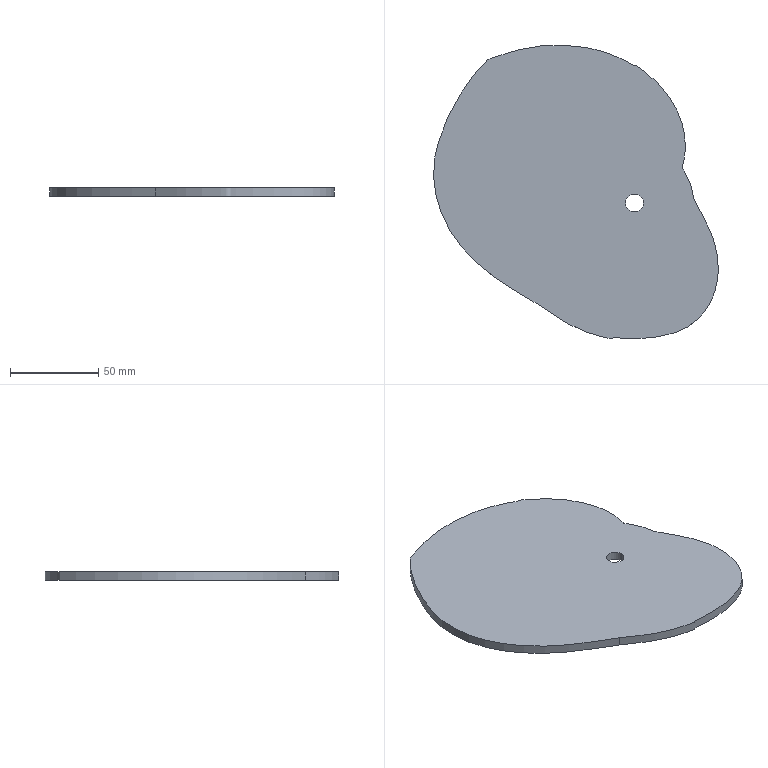Part | SolidWorks | features CurveInFile 1, Extrusion 1, ICE 1 | 1 solid | 6 faces | box 161.75 x 166.846 x 5 mm | volume 99438 mm3 | cylinder 2 | spline 2 | plane 2 | commonest cylinder face diameters 10 x2